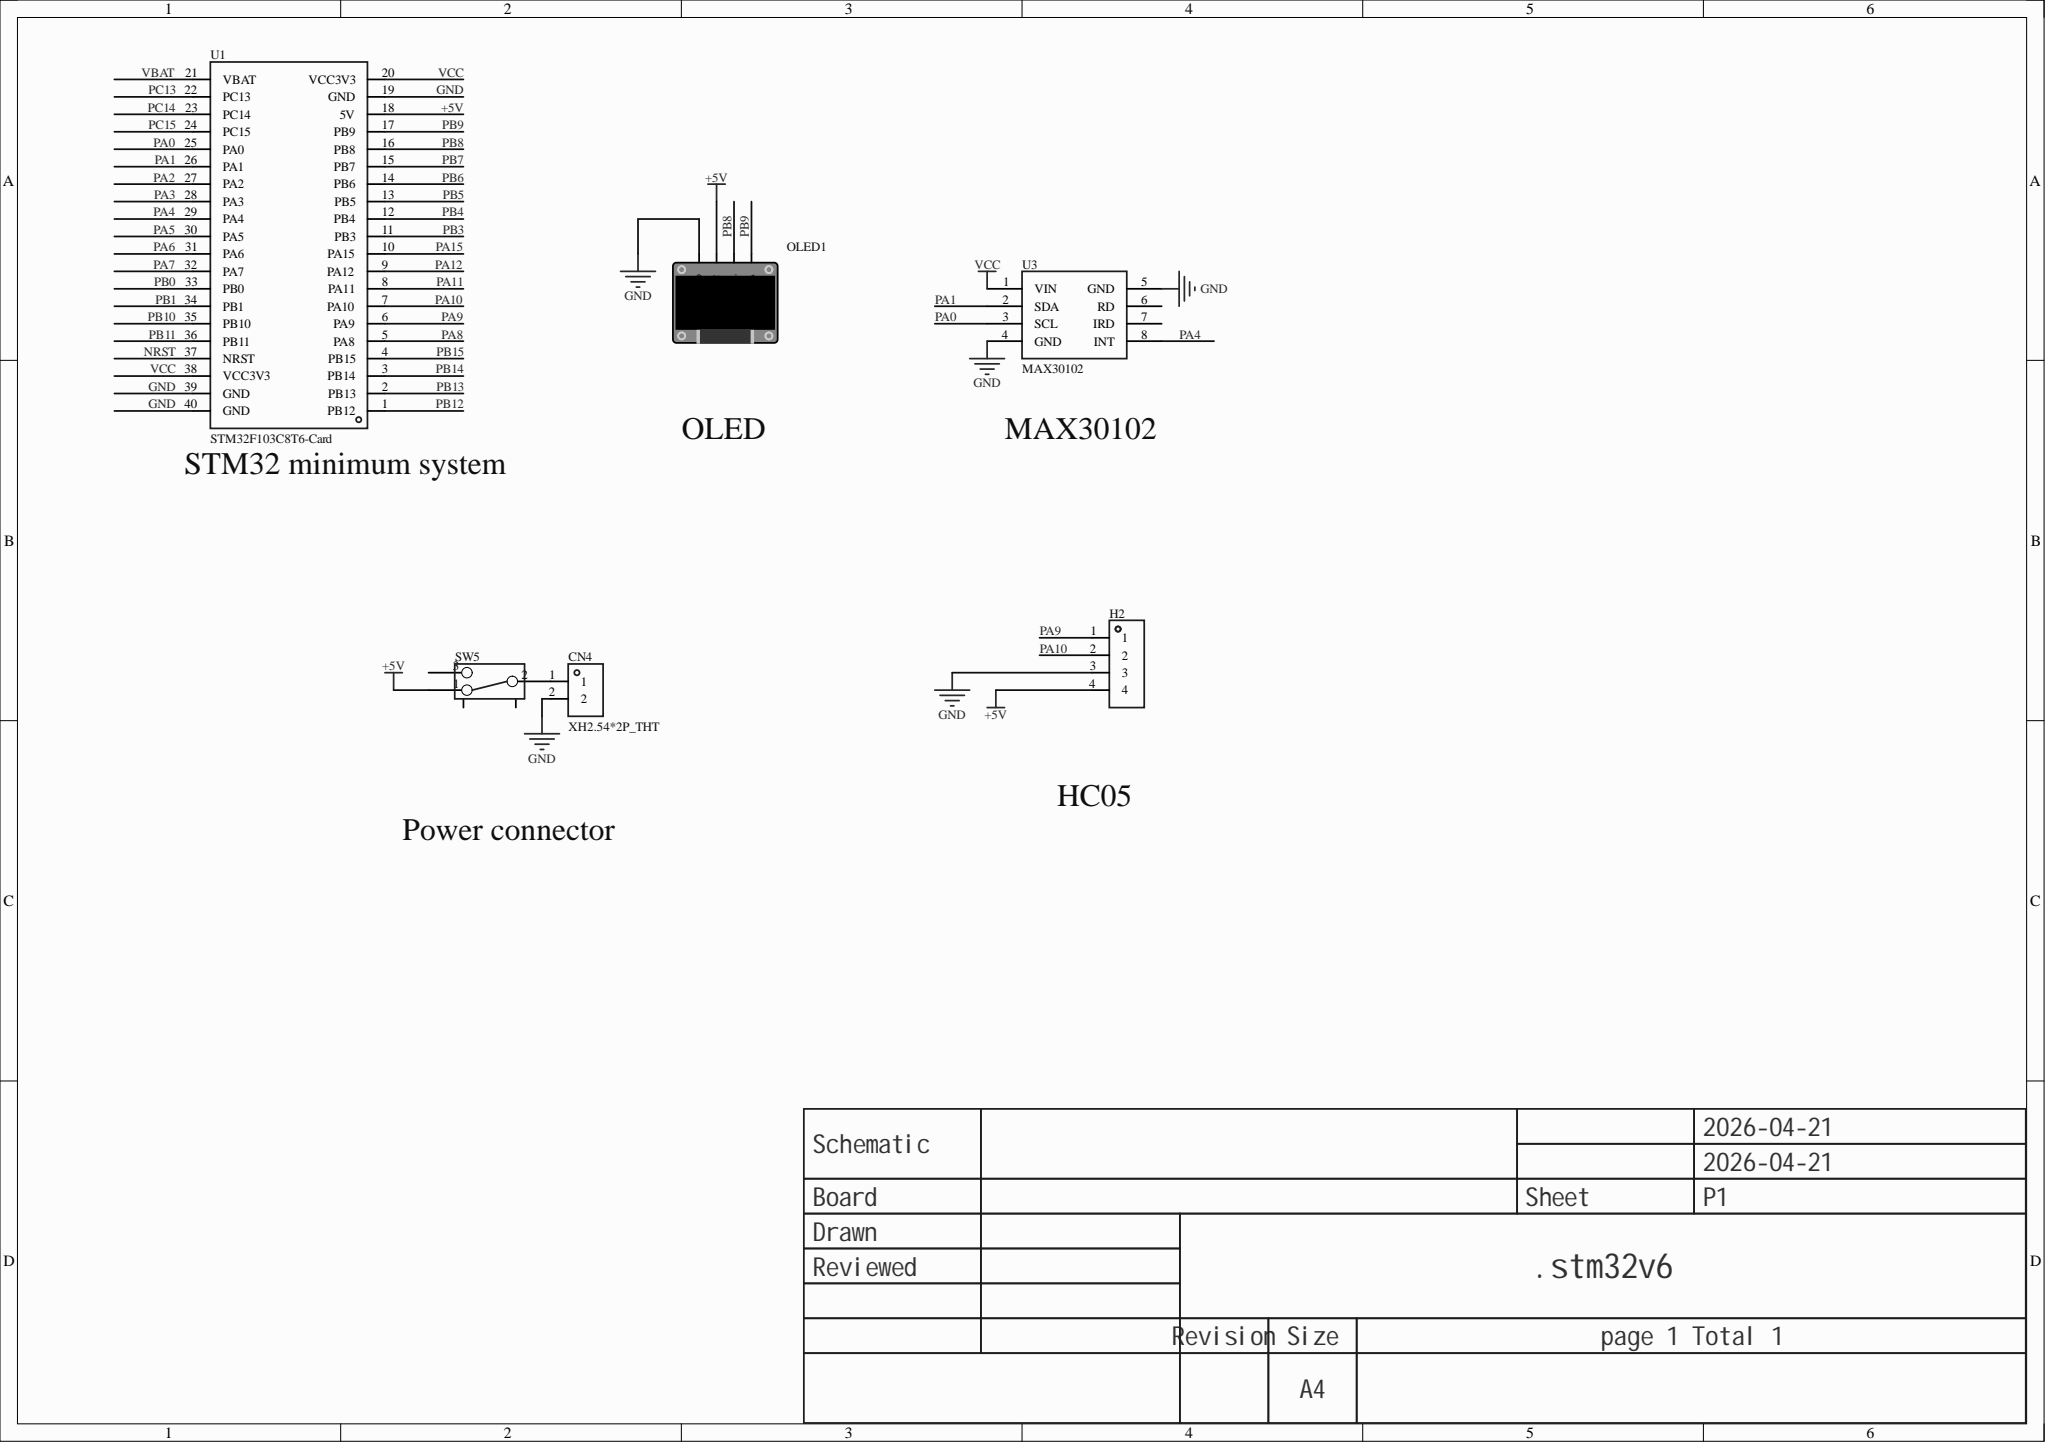Circuit board | Altium Designer | 6 parts | 11 nets
Bill of materials:
Comment,Description,Designator,Footprint,LibRef,Quantity
"XH2.54*2P_THT","","CN4","CONN-TH_2P-P2.50-XH2.54-2P","XH2.54*2P_直插","1"
"","","H2","HDR-TH_4P-P2.54-V-F","HDR-F_2.54_1x4P","1"
"","","OLED1","0.96OLED_4P","0.96OLED模块_4P","1"
"","","SW5","拨动开关","拨动开关_正","1"
"STM32F103C8T6-Card","","U1","CONN-TH_L53.3-W22.9_STM32F103C8T6-CARD","STM32F103C8T6-Card","1"
"MAX30102","","U3","MAX30102","MAX30102","1"
Netlist (Protel format):
[
CN4
CONN-TH_2P-P2.50-XH2.54-2P
XH2.54*2P_THT



]
[
H2
HDR-TH_4P-P2.54-V-F




]
[
OLED1
0.96OLED_4P




]
[
SW5
拨动开关




]
[
U1
CONN-TH_L53.3-W22.9_STM32F103C8T6-CARD
STM32F103C8T6-Card



]
[
U3
MAX30102
MAX30102



]
(
VCC
U1-20
U1-38
U3-1
)
(
PB9
OLED1-4
U1-17
)
(
PB8
OLED1-3
U1-16
)
(
PA10
H2-2
U1-7
)
(
PA9
H2-1
U1-6
)
(
PA4
U1-29
U3-8
)
(
PA1
U1-26
U3-2
)
(
PA0
U1-25
U3-3
)
(
NetCN4_1
CN4-1
SW5-2
)
(
GND
CN4-2
H2-3
OLED1-1
U1-19
U1-39
U1-40
U3-4
U3-5
)
(
+5V
H2-4
OLED1-2
SW5-1
U1-18
)